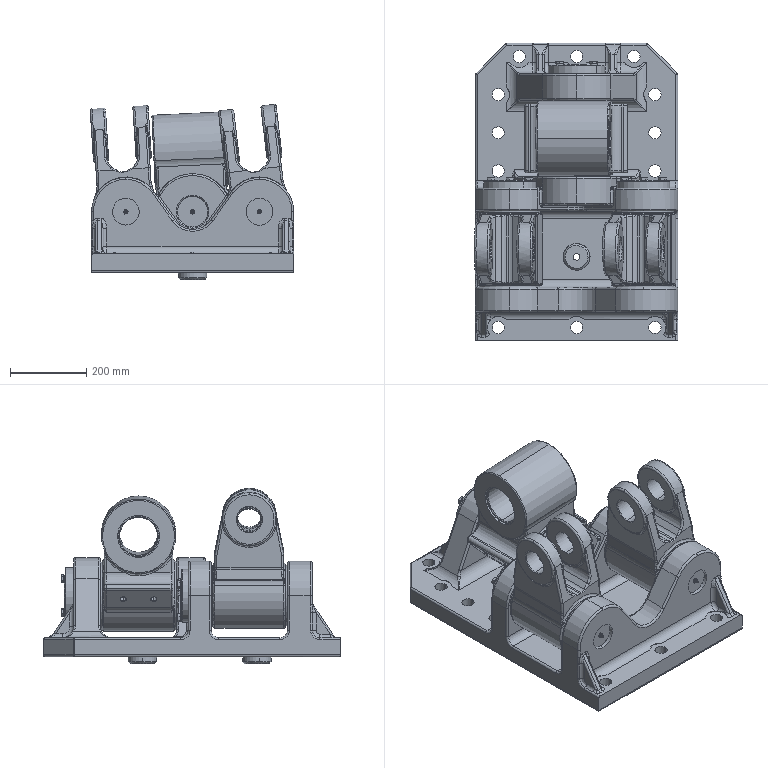Part | SolidWorks | features CompositeCurve 2 | 59 solids | 2083 faces | box 533.36 x 780 x 459.48 mm | volume 60459444 mm3 | cylinder 732 | plane 521 | cone 347 | torus 272 | spline 181 | sphere 30 | commonest cylinder face diameters 10 x145 3 x30 8 x30 12.2 x30 18.367 x30 14 x28